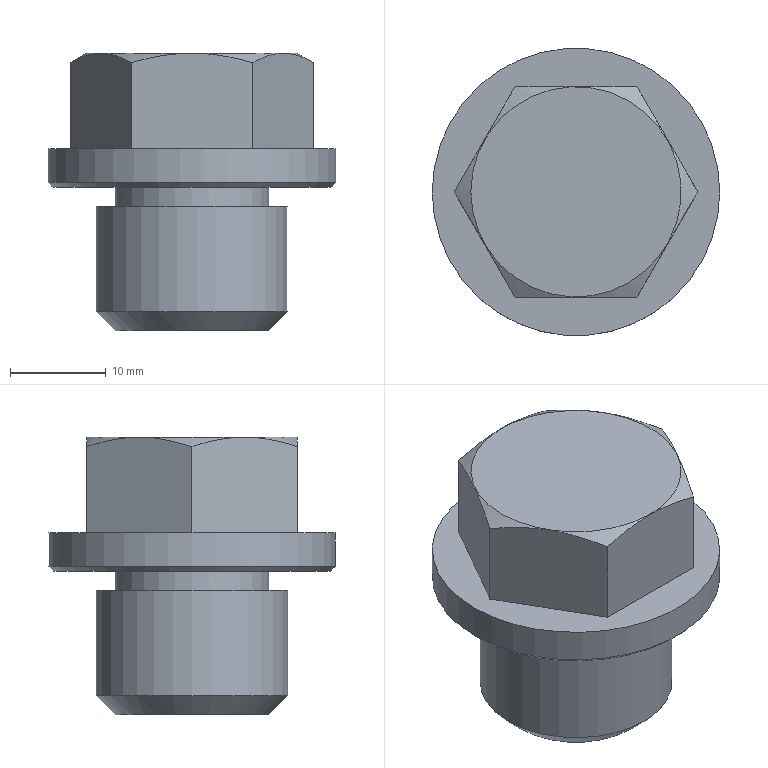Part | NX | features DATUM_CSYS 4, SKETCH 3, CHAMFER 2, SWP104 2, DATUM_PLANE 1, EXTRUDE 1 | 1 solid | 17 faces | box 30 x 30 x 29 mm | volume 11364 mm3 | plane 11 | cylinder 3 | cone 3 | commonest cylinder face diameters 16 x1 20 x1 30 x1
STEP:
#1=CARTESIAN_POINT('',(-8.,0.,0.));
#2=VERTEX_POINT('',#1);
#3=CARTESIAN_POINT('',(0.,0.,0.));
#4=DIRECTION('',(0.,0.,-1.));
#5=DIRECTION('',(-1.,0.,0.));
#6=AXIS2_PLACEMENT_3D('',#3,#4,#5);
#7=CIRCLE('',#6,8.);
#8=EDGE_CURVE('',#2,#2,#7,.T.);
#9=ORIENTED_EDGE('',*,*,#8,.T.);
#10=EDGE_LOOP('',(#9));
#11=FACE_BOUND('',#10,.T.);
#12=CARTESIAN_POINT('',(0.,0.,0.));
#13=DIRECTION('',(0.,0.,-1.));
#14=DIRECTION('',(-1.,0.,0.));
#15=AXIS2_PLACEMENT_3D('',#12,#13,#14);
#16=PLANE('',#15);
#17=ADVANCED_FACE('',(#11),#16,.T.);
#18=CARTESIAN_POINT('',(-10.,0.,2.));
#19=VERTEX_POINT('',#18);
#20=CARTESIAN_POINT('',(0.,0.,2.));
#21=DIRECTION('',(0.,0.,-1.));
#22=DIRECTION('',(-1.,0.,0.));
#23=AXIS2_PLACEMENT_3D('',#20,#21,#22);
#24=CIRCLE('',#23,10.);
#25=EDGE_CURVE('',#19,#19,#24,.F.);
#26=ORIENTED_EDGE('',*,*,#25,.T.);
#27=EDGE_LOOP('',(#26));
#28=FACE_BOUND('',#27,.T.);
#29=CARTESIAN_POINT('',(-10.,0.,13.));
#30=VERTEX_POINT('',#29);
#31=CARTESIAN_POINT('',(0.,0.,13.));
#32=DIRECTION('',(0.,0.,-1.));
#33=DIRECTION('',(-1.,0.,0.));
#34=AXIS2_PLACEMENT_3D('',#31,#32,#33);
#35=CIRCLE('',#34,10.);
#36=EDGE_CURVE('',#30,#30,#35,.T.);
#37=ORIENTED_EDGE('',*,*,#36,.T.);
#38=EDGE_LOOP('',(#37));
#39=FACE_BOUND('',#38,.T.);
#40=CARTESIAN_POINT('',(0.,0.,0.));
#41=DIRECTION('',(0.,0.,-1.));
#42=DIRECTION('',(-1.,0.,0.));
#43=AXIS2_PLACEMENT_3D('',#40,#41,#42);
#44=CYLINDRICAL_SURFACE('',#43,10.);
#45=ADVANCED_FACE('',(#28,#39),#44,.T.);
#46=CARTESIAN_POINT('',(-8.,0.,13.));
#47=VERTEX_POINT('',#46);
#48=CARTESIAN_POINT('',(0.,0.,13.));
#49=DIRECTION('',(0.,0.,-1.));
#50=DIRECTION('',(-1.,0.,0.));
#51=AXIS2_PLACEMENT_3D('',#48,#49,#50);
#52=CIRCLE('',#51,8.);
#53=EDGE_CURVE('',#47,#47,#52,.T.);
#54=ORIENTED_EDGE('',*,*,#53,.T.);
#55=EDGE_LOOP('',(#54));
#56=FACE_BOUND('',#55,.T.);
#57=ORIENTED_EDGE('',*,*,#36,.F.);
#58=EDGE_LOOP('',(#57));
#59=FACE_BOUND('',#58,.T.);
#60=CARTESIAN_POINT('',(0.,10.,13.));
#61=DIRECTION('',(0.,0.,1.));
#62=DIRECTION('',(1.,0.,0.));
#63=AXIS2_PLACEMENT_3D('',#60,#61,#62);
#64=PLANE('',#63);
#65=ADVANCED_FACE('',(#56,#59),#64,.T.);
#66=CARTESIAN_POINT('',(-8.,0.,15.));
#67=VERTEX_POINT('',#66);
#68=CARTESIAN_POINT('',(0.,0.,15.));
#69=DIRECTION('',(0.,0.,-1.));
#70=DIRECTION('',(-1.,0.,0.));
#71=AXIS2_PLACEMENT_3D('',#68,#69,#70);
#72=CIRCLE('',#71,8.);
#73=EDGE_CURVE('',#67,#67,#72,.T.);
#74=ORIENTED_EDGE('',*,*,#73,.T.);
#75=EDGE_LOOP('',(#74));
#76=FACE_BOUND('',#75,.T.);
#77=ORIENTED_EDGE('',*,*,#53,.F.);
#78=EDGE_LOOP('',(#77));
#79=FACE_BOUND('',#78,.T.);
#80=CARTESIAN_POINT('',(0.,0.,0.));
#81=DIRECTION('',(0.,0.,-1.));
#82=DIRECTION('',(-1.,0.,0.));
#83=AXIS2_PLACEMENT_3D('',#80,#81,#82);
#84=CYLINDRICAL_SURFACE('',#83,8.);
#85=ADVANCED_FACE('',(#76,#79),#84,.T.);
#86=CARTESIAN_POINT('',(-14.5,0.,15.));
#87=VERTEX_POINT('',#86);
#88=CARTESIAN_POINT('',(0.,0.,15.));
#89=DIRECTION('',(0.,0.,-1.));
#90=DIRECTION('',(-1.,0.,0.));
#91=AXIS2_PLACEMENT_3D('',#88,#89,#90);
#92=CIRCLE('',#91,14.5);
#93=EDGE_CURVE('',#87,#87,#92,.T.);
#94=ORIENTED_EDGE('',*,*,#93,.T.);
#95=EDGE_LOOP('',(#94));
#96=FACE_BOUND('',#95,.T.);
#97=ORIENTED_EDGE('',*,*,#73,.F.);
#98=EDGE_LOOP('',(#97));
#99=FACE_BOUND('',#98,.T.);
#100=CARTESIAN_POINT('',(0.,8.,15.));
#101=DIRECTION('',(0.,0.,-1.));
#102=DIRECTION('',(-1.,0.,0.));
#103=AXIS2_PLACEMENT_3D('',#100,#101,#102);
#104=PLANE('',#103);
#105=ADVANCED_FACE('',(#96,#99),#104,.T.);
#106=CARTESIAN_POINT('',(-15.,0.,15.5));
#107=VERTEX_POINT('',#106);
#108=CARTESIAN_POINT('',(0.,0.,15.5));
#109=DIRECTION('',(0.,0.,-1.));
#110=DIRECTION('',(-1.,0.,0.));
#111=AXIS2_PLACEMENT_3D('',#108,#109,#110);
#112=CIRCLE('',#111,15.);
#113=EDGE_CURVE('',#107,#107,#112,.F.);
#114=ORIENTED_EDGE('',*,*,#113,.T.);
#115=EDGE_LOOP('',(#114));
#116=FACE_BOUND('',#115,.T.);
#117=CARTESIAN_POINT('',(-15.,0.,19.));
#118=VERTEX_POINT('',#117);
#119=CARTESIAN_POINT('',(0.,0.,19.));
#120=DIRECTION('',(0.,0.,-1.));
#121=DIRECTION('',(-1.,0.,0.));
#122=AXIS2_PLACEMENT_3D('',#119,#120,#121);
#123=CIRCLE('',#122,15.);
#124=EDGE_CURVE('',#118,#118,#123,.T.);
#125=ORIENTED_EDGE('',*,*,#124,.T.);
#126=EDGE_LOOP('',(#125));
#127=FACE_BOUND('',#126,.T.);
#128=CARTESIAN_POINT('',(0.,0.,0.));
#129=DIRECTION('',(0.,0.,-1.));
#130=DIRECTION('',(-1.,0.,0.));
#131=AXIS2_PLACEMENT_3D('',#128,#129,#130);
#132=CYLINDRICAL_SURFACE('',#131,15.);
#133=ADVANCED_FACE('',(#116,#127),#132,.T.);
#134=CARTESIAN_POINT('',(-6.351,11.,19.));
#135=VERTEX_POINT('',#134);
#136=CARTESIAN_POINT('',(-12.702,0.,19.));
#137=VERTEX_POINT('',#136);
#138=CARTESIAN_POINT('',(-6.351,11.,19.));
#139=DIRECTION('',(-0.5,-0.866,0.));
#140=VECTOR('',#139,1000.);
#141=LINE('',#138,#140);
#142=EDGE_CURVE('',#135,#137,#141,.T.);
#143=ORIENTED_EDGE('',*,*,#142,.F.);
#144=CARTESIAN_POINT('',(6.351,11.,19.));
#145=VERTEX_POINT('',#144);
#146=CARTESIAN_POINT('',(6.351,11.,19.));
#147=DIRECTION('',(-1.,0.,0.));
#148=VECTOR('',#147,1000.);
#149=LINE('',#146,#148);
#150=EDGE_CURVE('',#145,#135,#149,.T.);
#151=ORIENTED_EDGE('',*,*,#150,.F.);
#152=CARTESIAN_POINT('',(12.702,0.,19.));
#153=VERTEX_POINT('',#152);
#154=CARTESIAN_POINT('',(12.702,0.,19.));
#155=DIRECTION('',(-0.5,0.866,0.));
#156=VECTOR('',#155,1000.);
#157=LINE('',#154,#156);
#158=EDGE_CURVE('',#153,#145,#157,.T.);
#159=ORIENTED_EDGE('',*,*,#158,.F.);
#160=CARTESIAN_POINT('',(6.351,-11.,19.));
#161=VERTEX_POINT('',#160);
#162=CARTESIAN_POINT('',(6.351,-11.,19.));
#163=DIRECTION('',(0.5,0.866,0.));
#164=VECTOR('',#163,1000.);
#165=LINE('',#162,#164);
#166=EDGE_CURVE('',#161,#153,#165,.T.);
#167=ORIENTED_EDGE('',*,*,#166,.F.);
#168=CARTESIAN_POINT('',(-6.351,-11.,19.));
#169=VERTEX_POINT('',#168);
#170=CARTESIAN_POINT('',(-6.351,-11.,19.));
#171=DIRECTION('',(1.,0.,0.));
#172=VECTOR('',#171,1000.);
#173=LINE('',#170,#172);
#174=EDGE_CURVE('',#169,#161,#173,.T.);
#175=ORIENTED_EDGE('',*,*,#174,.F.);
#176=CARTESIAN_POINT('',(-12.702,0.,19.));
#177=DIRECTION('',(0.5,-0.866,0.));
#178=VECTOR('',#177,1000.);
#179=LINE('',#176,#178);
#180=EDGE_CURVE('',#137,#169,#179,.T.);
#181=ORIENTED_EDGE('',*,*,#180,.F.);
#182=EDGE_LOOP('',(#143,#151,#159,#167,#175,#181));
#183=FACE_BOUND('',#182,.T.);
#184=ORIENTED_EDGE('',*,*,#124,.F.);
#185=EDGE_LOOP('',(#184));
#186=FACE_BOUND('',#185,.T.);
#187=CARTESIAN_POINT('',(0.,15.,19.));
#188=DIRECTION('',(0.,0.,1.));
#189=DIRECTION('',(1.,0.,0.));
#190=AXIS2_PLACEMENT_3D('',#187,#188,#189);
#191=PLANE('',#190);
#192=ADVANCED_FACE('',(#183,#186),#191,.T.);
#193=CARTESIAN_POINT('',(-12.702,0.,28.));
#194=VERTEX_POINT('',#193);
#195=CARTESIAN_POINT('',(-12.702,0.,29.));
#196=DIRECTION('',(0.,0.,-1.));
#197=VECTOR('',#196,1000.);
#198=LINE('',#195,#197);
#199=EDGE_CURVE('',#194,#137,#198,.T.);
#200=ORIENTED_EDGE('',*,*,#199,.F.);
#201=CARTESIAN_POINT('',(-6.351,11.,28.));
#202=VERTEX_POINT('',#201);
#203=CARTESIAN_POINT('',(-12.702,0.,28.));
#204=CARTESIAN_POINT('',(-11.665,1.796,28.599));
#205=CARTESIAN_POINT('',(-9.538,5.48,29.366));
#206=CARTESIAN_POINT('',(-7.389,9.202,28.599));
#207=CARTESIAN_POINT('',(-6.351,11.,28.));
#208=B_SPLINE_CURVE_WITH_KNOTS('',3,(#203,#204,#205,#206,#207),.UNSPECIFIED.,.F.,.F.,(4,1,4),(0.000000238,0.006414,0.01283),.UNSPECIFIED.);
#209=EDGE_CURVE('',#194,#202,#208,.T.);
#210=ORIENTED_EDGE('',*,*,#209,.T.);
#211=CARTESIAN_POINT('',(-6.351,11.,29.));
#212=DIRECTION('',(0.,0.,-1.));
#213=VECTOR('',#212,1000.);
#214=LINE('',#211,#213);
#215=EDGE_CURVE('',#202,#135,#214,.T.);
#216=ORIENTED_EDGE('',*,*,#215,.T.);
#217=ORIENTED_EDGE('',*,*,#142,.T.);
#218=EDGE_LOOP('',(#200,#210,#216,#217));
#219=FACE_BOUND('',#218,.T.);
#220=CARTESIAN_POINT('',(-6.351,11.,29.));
#221=DIRECTION('',(0.866,-0.5,0.));
#222=DIRECTION('',(0.5,0.866,0.));
#223=AXIS2_PLACEMENT_3D('',#220,#221,#222);
#224=PLANE('',#223);
#225=ADVANCED_FACE('',(#219),#224,.F.);
#226=CARTESIAN_POINT('',(-6.351,-11.,28.));
#227=VERTEX_POINT('',#226);
#228=CARTESIAN_POINT('',(-6.351,-11.,29.));
#229=DIRECTION('',(0.,0.,-1.));
#230=VECTOR('',#229,1000.);
#231=LINE('',#228,#230);
#232=EDGE_CURVE('',#227,#169,#231,.T.);
#233=ORIENTED_EDGE('',*,*,#232,.F.);
#234=CARTESIAN_POINT('',(-6.351,-11.,28.));
#235=CARTESIAN_POINT('',(-7.388,-9.204,28.599));
#236=CARTESIAN_POINT('',(-9.515,-5.52,29.366));
#237=CARTESIAN_POINT('',(-11.663,-1.798,28.599));
#238=CARTESIAN_POINT('',(-12.702,0.,28.));
#239=B_SPLINE_CURVE_WITH_KNOTS('',3,(#234,#235,#236,#237,#238),.UNSPECIFIED.,.F.,.F.,(4,1,4),(0.000000238,0.006414,0.01283),.UNSPECIFIED.);
#240=EDGE_CURVE('',#227,#194,#239,.T.);
#241=ORIENTED_EDGE('',*,*,#240,.T.);
#242=ORIENTED_EDGE('',*,*,#199,.T.);
#243=ORIENTED_EDGE('',*,*,#180,.T.);
#244=EDGE_LOOP('',(#233,#241,#242,#243));
#245=FACE_BOUND('',#244,.T.);
#246=CARTESIAN_POINT('',(-12.702,0.,29.));
#247=DIRECTION('',(0.866,0.5,0.));
#248=DIRECTION('',(-0.5,0.866,0.));
#249=AXIS2_PLACEMENT_3D('',#246,#247,#248);
#250=PLANE('',#249);
#251=ADVANCED_FACE('',(#245),#250,.F.);
#252=CARTESIAN_POINT('',(6.351,-11.,28.));
#253=VERTEX_POINT('',#252);
#254=CARTESIAN_POINT('',(6.351,-11.,29.));
#255=DIRECTION('',(0.,0.,-1.));
#256=VECTOR('',#255,1000.);
#257=LINE('',#254,#256);
#258=EDGE_CURVE('',#253,#161,#257,.T.);
#259=ORIENTED_EDGE('',*,*,#258,.F.);
#260=CARTESIAN_POINT('',(-6.351,-11.,28.));
#261=CARTESIAN_POINT('',(-4.284,-11.,28.597));
#262=CARTESIAN_POINT('',(-0.002802,-11.,29.37));
#263=CARTESIAN_POINT('',(4.298,-11.,28.593));
#264=CARTESIAN_POINT('',(6.351,-11.,28.));
#265=B_SPLINE_CURVE_WITH_KNOTS('',3,(#260,#261,#262,#263,#264),.UNSPECIFIED.,.F.,.F.,(4,1,4),(0.01133,0.01775,0.02418),.UNSPECIFIED.);
#266=EDGE_CURVE('',#253,#227,#265,.F.);
#267=ORIENTED_EDGE('',*,*,#266,.T.);
#268=ORIENTED_EDGE('',*,*,#232,.T.);
#269=ORIENTED_EDGE('',*,*,#174,.T.);
#270=EDGE_LOOP('',(#259,#267,#268,#269));
#271=FACE_BOUND('',#270,.T.);
#272=CARTESIAN_POINT('',(-6.351,-11.,29.));
#273=DIRECTION('',(0.,1.,0.));
#274=DIRECTION('',(-1.,0.,0.));
#275=AXIS2_PLACEMENT_3D('',#272,#273,#274);
#276=PLANE('',#275);
#277=ADVANCED_FACE('',(#271),#276,.F.);
#278=CARTESIAN_POINT('',(12.702,0.,28.));
#279=VERTEX_POINT('',#278);
#280=CARTESIAN_POINT('',(12.702,0.,29.));
#281=DIRECTION('',(0.,0.,-1.));
#282=VECTOR('',#281,1000.);
#283=LINE('',#280,#282);
#284=EDGE_CURVE('',#279,#153,#283,.T.);
#285=ORIENTED_EDGE('',*,*,#284,.F.);
#286=CARTESIAN_POINT('',(12.702,0.,28.));
#287=CARTESIAN_POINT('',(11.665,-1.796,28.599));
#288=CARTESIAN_POINT('',(9.538,-5.48,29.366));
#289=CARTESIAN_POINT('',(7.389,-9.202,28.599));
#290=CARTESIAN_POINT('',(6.351,-11.,28.));
#291=B_SPLINE_CURVE_WITH_KNOTS('',3,(#286,#287,#288,#289,#290),.UNSPECIFIED.,.F.,.F.,(4,1,4),(0.000000238,0.006414,0.01283),.UNSPECIFIED.);
#292=EDGE_CURVE('',#279,#253,#291,.T.);
#293=ORIENTED_EDGE('',*,*,#292,.T.);
#294=ORIENTED_EDGE('',*,*,#258,.T.);
#295=ORIENTED_EDGE('',*,*,#166,.T.);
#296=EDGE_LOOP('',(#285,#293,#294,#295));
#297=FACE_BOUND('',#296,.T.);
#298=CARTESIAN_POINT('',(6.351,-11.,29.));
#299=DIRECTION('',(-0.866,0.5,0.));
#300=DIRECTION('',(-0.5,-0.866,0.));
#301=AXIS2_PLACEMENT_3D('',#298,#299,#300);
#302=PLANE('',#301);
#303=ADVANCED_FACE('',(#297),#302,.F.);
#304=CARTESIAN_POINT('',(6.351,11.,28.));
#305=VERTEX_POINT('',#304);
#306=CARTESIAN_POINT('',(6.351,11.,29.));
#307=DIRECTION('',(0.,0.,-1.));
#308=VECTOR('',#307,1000.);
#309=LINE('',#306,#308);
#310=EDGE_CURVE('',#305,#145,#309,.T.);
#311=ORIENTED_EDGE('',*,*,#310,.F.);
#312=CARTESIAN_POINT('',(6.351,11.,28.));
#313=CARTESIAN_POINT('',(7.388,9.204,28.599));
#314=CARTESIAN_POINT('',(9.515,5.52,29.366));
#315=CARTESIAN_POINT('',(11.663,1.798,28.599));
#316=CARTESIAN_POINT('',(12.702,0.,28.));
#317=B_SPLINE_CURVE_WITH_KNOTS('',3,(#312,#313,#314,#315,#316),.UNSPECIFIED.,.F.,.F.,(4,1,4),(0.000000238,0.006414,0.01283),.UNSPECIFIED.);
#318=EDGE_CURVE('',#305,#279,#317,.T.);
#319=ORIENTED_EDGE('',*,*,#318,.T.);
#320=ORIENTED_EDGE('',*,*,#284,.T.);
#321=ORIENTED_EDGE('',*,*,#158,.T.);
#322=EDGE_LOOP('',(#311,#319,#320,#321));
#323=FACE_BOUND('',#322,.T.);
#324=CARTESIAN_POINT('',(12.702,0.,29.));
#325=DIRECTION('',(-0.866,-0.5,0.));
#326=DIRECTION('',(0.5,-0.866,0.));
#327=AXIS2_PLACEMENT_3D('',#324,#325,#326);
#328=PLANE('',#327);
#329=ADVANCED_FACE('',(#323),#328,.F.);
#330=ORIENTED_EDGE('',*,*,#215,.F.);
#331=CARTESIAN_POINT('',(-6.351,11.,28.));
#332=CARTESIAN_POINT('',(-4.284,11.,28.597));
#333=CARTESIAN_POINT('',(-0.002802,11.,29.37));
#334=CARTESIAN_POINT('',(4.298,11.,28.593));
#335=CARTESIAN_POINT('',(6.351,11.,28.));
#336=B_SPLINE_CURVE_WITH_KNOTS('',3,(#331,#332,#333,#334,#335),.UNSPECIFIED.,.F.,.F.,(4,1,4),(0.01133,0.01775,0.02418),.UNSPECIFIED.);
#337=EDGE_CURVE('',#202,#305,#336,.T.);
#338=ORIENTED_EDGE('',*,*,#337,.T.);
#339=ORIENTED_EDGE('',*,*,#310,.T.);
#340=ORIENTED_EDGE('',*,*,#150,.T.);
#341=EDGE_LOOP('',(#330,#338,#339,#340));
#342=FACE_BOUND('',#341,.T.);
#343=CARTESIAN_POINT('',(6.351,11.,29.));
#344=DIRECTION('',(0.,-1.,0.));
#345=DIRECTION('',(0.,0.,-1.));
#346=AXIS2_PLACEMENT_3D('',#343,#344,#345);
#347=PLANE('',#346);
#348=ADVANCED_FACE('',(#342),#347,.F.);
#349=CARTESIAN_POINT('',(-10.97,0.,29.));
#350=VERTEX_POINT('',#349);
#351=CARTESIAN_POINT('',(0.,0.,29.));
#352=DIRECTION('',(0.,0.,-1.));
#353=DIRECTION('',(-1.,0.,0.));
#354=AXIS2_PLACEMENT_3D('',#351,#352,#353);
#355=CIRCLE('',#354,10.97);
#356=EDGE_CURVE('',#350,#350,#355,.T.);
#357=ORIENTED_EDGE('',*,*,#356,.T.);
#358=EDGE_LOOP('',(#357));
#359=FACE_BOUND('',#358,.T.);
#360=ORIENTED_EDGE('',*,*,#240,.F.);
#361=ORIENTED_EDGE('',*,*,#266,.F.);
#362=ORIENTED_EDGE('',*,*,#292,.F.);
#363=ORIENTED_EDGE('',*,*,#318,.F.);
#364=ORIENTED_EDGE('',*,*,#337,.F.);
#365=ORIENTED_EDGE('',*,*,#209,.F.);
#366=EDGE_LOOP('',(#360,#361,#362,#363,#364,#365));
#367=FACE_BOUND('',#366,.T.);
#368=CARTESIAN_POINT('',(0.,0.,29.));
#369=DIRECTION('',(0.,0.,-1.));
#370=DIRECTION('',(-1.,0.,0.));
#371=AXIS2_PLACEMENT_3D('',#368,#369,#370);
#372=CONICAL_SURFACE('',#371,10.97,1.047);
#373=ADVANCED_FACE('',(#359,#367),#372,.T.);
#374=ORIENTED_EDGE('',*,*,#356,.F.);
#375=EDGE_LOOP('',(#374));
#376=FACE_BOUND('',#375,.T.);
#377=CARTESIAN_POINT('',(0.,0.,29.));
#378=DIRECTION('',(0.,0.,1.));
#379=DIRECTION('',(1.,0.,0.));
#380=AXIS2_PLACEMENT_3D('',#377,#378,#379);
#381=PLANE('',#380);
#382=ADVANCED_FACE('',(#376),#381,.T.);
#383=ORIENTED_EDGE('',*,*,#113,.F.);
#384=EDGE_LOOP('',(#383));
#385=FACE_BOUND('',#384,.T.);
#386=ORIENTED_EDGE('',*,*,#93,.F.);
#387=EDGE_LOOP('',(#386));
#388=FACE_BOUND('',#387,.T.);
#389=CARTESIAN_POINT('',(0.,0.,15.));
#390=DIRECTION('',(0.,0.,1.));
#391=DIRECTION('',(1.,0.,0.));
#392=AXIS2_PLACEMENT_3D('',#389,#390,#391);
#393=CONICAL_SURFACE('',#392,14.5,0.7854);
#394=ADVANCED_FACE('',(#385,#388),#393,.T.);
#395=ORIENTED_EDGE('',*,*,#25,.F.);
#396=EDGE_LOOP('',(#395));
#397=FACE_BOUND('',#396,.T.);
#398=ORIENTED_EDGE('',*,*,#8,.F.);
#399=EDGE_LOOP('',(#398));
#400=FACE_BOUND('',#399,.T.);
#401=CARTESIAN_POINT('',(0.,0.,0.));
#402=DIRECTION('',(0.,0.,1.));
#403=DIRECTION('',(1.,0.,0.));
#404=AXIS2_PLACEMENT_3D('',#401,#402,#403);
#405=CONICAL_SURFACE('',#404,8.,0.7854);
#406=ADVANCED_FACE('',(#397,#400),#405,.T.);
#407=CLOSED_SHELL('',(#17,#45,#65,#85,#105,#133,#192,#225,#251,#277,#303,#329,#348,#373,#382,#394,#406));
#408=MANIFOLD_SOLID_BREP('',#407);
#409=(LENGTH_UNIT()NAMED_UNIT(*)SI_UNIT(.MILLI.,.METRE.));
#410=UNCERTAINTY_MEASURE_WITH_UNIT(LENGTH_MEASURE(0.0508),#409,'','');
#411=(NAMED_UNIT(*)PLANE_ANGLE_UNIT()SI_UNIT($,.RADIAN.));
#412=(NAMED_UNIT(*)SI_UNIT($,.STERADIAN.)SOLID_ANGLE_UNIT());
#413=(GEOMETRIC_REPRESENTATION_CONTEXT(3)GLOBAL_UNCERTAINTY_ASSIGNED_CONTEXT((#410))GLOBAL_UNIT_ASSIGNED_CONTEXT((#409,#411,#412))REPRESENTATION_CONTEXT('',''));
#414=ADVANCED_BREP_SHAPE_REPRESENTATION('',(#408),#413);